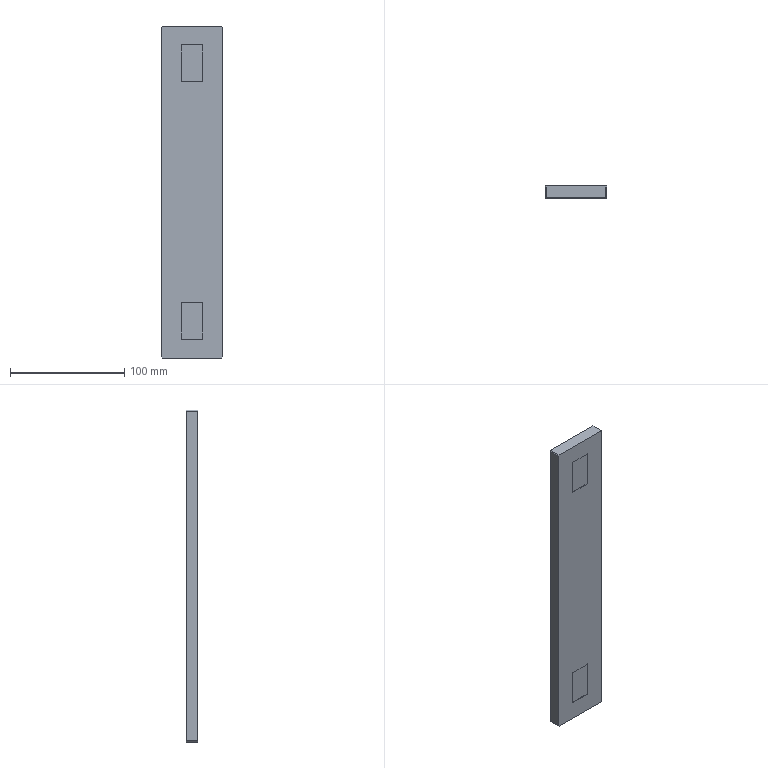Part | SolidWorks | 1 solid | 25 faces | box 54 x 10 x 290 mm | volume 145188 mm3 | plane 25
STEP:
#1=CARTESIAN_POINT('',(9.25,0.,-96.5));
#2=VERTEX_POINT('',#1);
#3=CARTESIAN_POINT('',(9.25,0.5,-96.5));
#4=VERTEX_POINT('',#3);
#5=CARTESIAN_POINT('',(9.25,-193.885,-96.5));
#6=DIRECTION('',(0.,1.,0.));
#7=VECTOR('',#6,1000.);
#8=LINE('',#5,#7);
#9=EDGE_CURVE('',#2,#4,#8,.T.);
#10=ORIENTED_EDGE('',*,*,#9,.T.);
#11=CARTESIAN_POINT('',(9.25,0.5,-128.5));
#12=VERTEX_POINT('',#11);
#13=CARTESIAN_POINT('',(9.25,0.5,128.5));
#14=DIRECTION('',(0.,0.,1.));
#15=VECTOR('',#14,1000.);
#16=LINE('',#13,#15);
#17=EDGE_CURVE('',#12,#4,#16,.T.);
#18=ORIENTED_EDGE('',*,*,#17,.F.);
#19=CARTESIAN_POINT('',(9.25,0.,-128.5));
#20=VERTEX_POINT('',#19);
#21=CARTESIAN_POINT('',(9.25,0.5,-128.5));
#22=DIRECTION('',(0.,-1.,0.));
#23=VECTOR('',#22,1000.);
#24=LINE('',#21,#23);
#25=EDGE_CURVE('',#12,#20,#24,.T.);
#26=ORIENTED_EDGE('',*,*,#25,.T.);
#27=CARTESIAN_POINT('',(9.25,0.,128.5));
#28=DIRECTION('',(0.,0.,1.));
#29=VECTOR('',#28,1000.);
#30=LINE('',#27,#29);
#31=EDGE_CURVE('',#20,#2,#30,.T.);
#32=ORIENTED_EDGE('',*,*,#31,.T.);
#33=EDGE_LOOP('',(#10,#18,#26,#32));
#34=FACE_OUTER_BOUND('',#33,.T.);
#35=CARTESIAN_POINT('',(9.25,0.5,128.5));
#36=DIRECTION('',(1.,0.,0.));
#37=DIRECTION('',(0.,0.,-1.));
#38=AXIS2_PLACEMENT_3D('',#35,#36,#37);
#39=PLANE('',#38);
#40=ADVANCED_FACE('',(#34),#39,.F.);
#41=CARTESIAN_POINT('',(9.25,0.,96.5));
#42=VERTEX_POINT('',#41);
#43=CARTESIAN_POINT('',(9.25,0.5,96.5));
#44=VERTEX_POINT('',#43);
#45=CARTESIAN_POINT('',(9.25,-193.885,96.5));
#46=DIRECTION('',(0.,1.,0.));
#47=VECTOR('',#46,1000.);
#48=LINE('',#45,#47);
#49=EDGE_CURVE('',#42,#44,#48,.T.);
#50=ORIENTED_EDGE('',*,*,#49,.F.);
#51=CARTESIAN_POINT('',(9.25,0.,128.5));
#52=VERTEX_POINT('',#51);
#53=CARTESIAN_POINT('',(9.25,0.,128.5));
#54=DIRECTION('',(0.,0.,1.));
#55=VECTOR('',#54,1000.);
#56=LINE('',#53,#55);
#57=EDGE_CURVE('',#42,#52,#56,.T.);
#58=ORIENTED_EDGE('',*,*,#57,.T.);
#59=CARTESIAN_POINT('',(9.25,0.5,128.5));
#60=VERTEX_POINT('',#59);
#61=CARTESIAN_POINT('',(9.25,0.5,128.5));
#62=DIRECTION('',(0.,-1.,0.));
#63=VECTOR('',#62,1000.);
#64=LINE('',#61,#63);
#65=EDGE_CURVE('',#60,#52,#64,.T.);
#66=ORIENTED_EDGE('',*,*,#65,.F.);
#67=CARTESIAN_POINT('',(9.25,0.5,128.5));
#68=DIRECTION('',(0.,0.,1.));
#69=VECTOR('',#68,1000.);
#70=LINE('',#67,#69);
#71=EDGE_CURVE('',#44,#60,#70,.T.);
#72=ORIENTED_EDGE('',*,*,#71,.F.);
#73=EDGE_LOOP('',(#50,#58,#66,#72));
#74=FACE_OUTER_BOUND('',#73,.T.);
#75=CARTESIAN_POINT('',(9.25,0.5,128.5));
#76=DIRECTION('',(1.,0.,0.));
#77=DIRECTION('',(0.,0.,-1.));
#78=AXIS2_PLACEMENT_3D('',#75,#76,#77);
#79=PLANE('',#78);
#80=ADVANCED_FACE('',(#74),#79,.F.);
#81=CARTESIAN_POINT('',(-9.25,0.,-96.5));
#82=VERTEX_POINT('',#81);
#83=CARTESIAN_POINT('',(-9.25,0.5,-96.5));
#84=VERTEX_POINT('',#83);
#85=CARTESIAN_POINT('',(-9.25,-193.885,-96.5));
#86=DIRECTION('',(0.,1.,0.));
#87=VECTOR('',#86,1000.);
#88=LINE('',#85,#87);
#89=EDGE_CURVE('',#82,#84,#88,.T.);
#90=ORIENTED_EDGE('',*,*,#89,.F.);
#91=CARTESIAN_POINT('',(-9.25,0.,-128.5));
#92=VERTEX_POINT('',#91);
#93=CARTESIAN_POINT('',(-9.25,0.,128.5));
#94=DIRECTION('',(0.,0.,-1.));
#95=VECTOR('',#94,1000.);
#96=LINE('',#93,#95);
#97=EDGE_CURVE('',#82,#92,#96,.T.);
#98=ORIENTED_EDGE('',*,*,#97,.T.);
#99=CARTESIAN_POINT('',(-9.25,0.5,-128.5));
#100=VERTEX_POINT('',#99);
#101=CARTESIAN_POINT('',(-9.25,0.5,-128.5));
#102=DIRECTION('',(0.,-1.,0.));
#103=VECTOR('',#102,1000.);
#104=LINE('',#101,#103);
#105=EDGE_CURVE('',#100,#92,#104,.T.);
#106=ORIENTED_EDGE('',*,*,#105,.F.);
#107=CARTESIAN_POINT('',(-9.25,0.5,128.5));
#108=DIRECTION('',(0.,0.,-1.));
#109=VECTOR('',#108,1000.);
#110=LINE('',#107,#109);
#111=EDGE_CURVE('',#84,#100,#110,.T.);
#112=ORIENTED_EDGE('',*,*,#111,.F.);
#113=EDGE_LOOP('',(#90,#98,#106,#112));
#114=FACE_OUTER_BOUND('',#113,.T.);
#115=CARTESIAN_POINT('',(-9.25,0.5,128.5));
#116=DIRECTION('',(-1.,0.,0.));
#117=DIRECTION('',(0.,0.,1.));
#118=AXIS2_PLACEMENT_3D('',#115,#116,#117);
#119=PLANE('',#118);
#120=ADVANCED_FACE('',(#114),#119,.F.);
#121=CARTESIAN_POINT('',(-9.25,0.,96.5));
#122=VERTEX_POINT('',#121);
#123=CARTESIAN_POINT('',(-9.25,0.5,96.5));
#124=VERTEX_POINT('',#123);
#125=CARTESIAN_POINT('',(-9.25,-193.885,96.5));
#126=DIRECTION('',(0.,1.,0.));
#127=VECTOR('',#126,1000.);
#128=LINE('',#125,#127);
#129=EDGE_CURVE('',#122,#124,#128,.T.);
#130=ORIENTED_EDGE('',*,*,#129,.T.);
#131=CARTESIAN_POINT('',(-9.25,0.5,128.5));
#132=VERTEX_POINT('',#131);
#133=CARTESIAN_POINT('',(-9.25,0.5,128.5));
#134=DIRECTION('',(0.,0.,-1.));
#135=VECTOR('',#134,1000.);
#136=LINE('',#133,#135);
#137=EDGE_CURVE('',#132,#124,#136,.T.);
#138=ORIENTED_EDGE('',*,*,#137,.F.);
#139=CARTESIAN_POINT('',(-9.25,0.,128.5));
#140=VERTEX_POINT('',#139);
#141=CARTESIAN_POINT('',(-9.25,0.5,128.5));
#142=DIRECTION('',(0.,-1.,0.));
#143=VECTOR('',#142,1000.);
#144=LINE('',#141,#143);
#145=EDGE_CURVE('',#132,#140,#144,.T.);
#146=ORIENTED_EDGE('',*,*,#145,.T.);
#147=CARTESIAN_POINT('',(-9.25,0.,128.5));
#148=DIRECTION('',(0.,0.,-1.));
#149=VECTOR('',#148,1000.);
#150=LINE('',#147,#149);
#151=EDGE_CURVE('',#140,#122,#150,.T.);
#152=ORIENTED_EDGE('',*,*,#151,.T.);
#153=EDGE_LOOP('',(#130,#138,#146,#152));
#154=FACE_OUTER_BOUND('',#153,.T.);
#155=CARTESIAN_POINT('',(-9.25,0.5,128.5));
#156=DIRECTION('',(-1.,0.,0.));
#157=DIRECTION('',(0.,0.,1.));
#158=AXIS2_PLACEMENT_3D('',#155,#156,#157);
#159=PLANE('',#158);
#160=ADVANCED_FACE('',(#154),#159,.F.);
#161=ORIENTED_EDGE('',*,*,#17,.T.);
#162=CARTESIAN_POINT('',(-9.25,0.5,-96.5));
#163=DIRECTION('',(1.,0.,0.));
#164=VECTOR('',#163,1000.);
#165=LINE('',#162,#164);
#166=EDGE_CURVE('',#84,#4,#165,.T.);
#167=ORIENTED_EDGE('',*,*,#166,.F.);
#168=ORIENTED_EDGE('',*,*,#111,.T.);
#169=CARTESIAN_POINT('',(-9.25,0.5,-128.5));
#170=DIRECTION('',(1.,0.,0.));
#171=VECTOR('',#170,1000.);
#172=LINE('',#169,#171);
#173=EDGE_CURVE('',#100,#12,#172,.T.);
#174=ORIENTED_EDGE('',*,*,#173,.T.);
#175=EDGE_LOOP('',(#161,#167,#168,#174));
#176=FACE_OUTER_BOUND('',#175,.T.);
#177=CARTESIAN_POINT('',(0.,0.5,0.));
#178=DIRECTION('',(0.,-1.,0.));
#179=DIRECTION('',(0.,0.,-1.));
#180=AXIS2_PLACEMENT_3D('',#177,#178,#179);
#181=PLANE('',#180);
#182=ADVANCED_FACE('',(#176),#181,.T.);
#183=ORIENTED_EDGE('',*,*,#137,.T.);
#184=CARTESIAN_POINT('',(-9.25,0.5,96.5));
#185=DIRECTION('',(-1.,0.,0.));
#186=VECTOR('',#185,1000.);
#187=LINE('',#184,#186);
#188=EDGE_CURVE('',#44,#124,#187,.T.);
#189=ORIENTED_EDGE('',*,*,#188,.F.);
#190=ORIENTED_EDGE('',*,*,#71,.T.);
#191=CARTESIAN_POINT('',(-9.25,0.5,128.5));
#192=DIRECTION('',(-1.,0.,0.));
#193=VECTOR('',#192,1000.);
#194=LINE('',#191,#193);
#195=EDGE_CURVE('',#60,#132,#194,.T.);
#196=ORIENTED_EDGE('',*,*,#195,.T.);
#197=EDGE_LOOP('',(#183,#189,#190,#196));
#198=FACE_OUTER_BOUND('',#197,.T.);
#199=CARTESIAN_POINT('',(0.,0.5,0.));
#200=DIRECTION('',(0.,-1.,0.));
#201=DIRECTION('',(0.,0.,-1.));
#202=AXIS2_PLACEMENT_3D('',#199,#200,#201);
#203=PLANE('',#202);
#204=ADVANCED_FACE('',(#198),#203,.T.);
#205=CARTESIAN_POINT('',(27.,0.,144.));
#206=VERTEX_POINT('',#205);
#207=CARTESIAN_POINT('',(27.,0.,-144.));
#208=VERTEX_POINT('',#207);
#209=CARTESIAN_POINT('',(27.,0.,-145.));
#210=DIRECTION('',(0.,0.,-1.));
#211=VECTOR('',#210,1000.);
#212=LINE('',#209,#211);
#213=EDGE_CURVE('',#206,#208,#212,.T.);
#214=ORIENTED_EDGE('',*,*,#213,.T.);
#215=CARTESIAN_POINT('',(27.,10.,-144.));
#216=VERTEX_POINT('',#215);
#217=CARTESIAN_POINT('',(27.,10.,-144.));
#218=DIRECTION('',(0.,1.,0.));
#219=VECTOR('',#218,1000.);
#220=LINE('',#217,#219);
#221=EDGE_CURVE('',#208,#216,#220,.T.);
#222=ORIENTED_EDGE('',*,*,#221,.T.);
#223=CARTESIAN_POINT('',(27.,10.,144.));
#224=VERTEX_POINT('',#223);
#225=CARTESIAN_POINT('',(27.,10.,-145.));
#226=DIRECTION('',(0.,0.,-1.));
#227=VECTOR('',#226,1000.);
#228=LINE('',#225,#227);
#229=EDGE_CURVE('',#224,#216,#228,.T.);
#230=ORIENTED_EDGE('',*,*,#229,.F.);
#231=CARTESIAN_POINT('',(27.,10.,144.));
#232=DIRECTION('',(0.,-1.,0.));
#233=VECTOR('',#232,1000.);
#234=LINE('',#231,#233);
#235=EDGE_CURVE('',#224,#206,#234,.T.);
#236=ORIENTED_EDGE('',*,*,#235,.T.);
#237=EDGE_LOOP('',(#214,#222,#230,#236));
#238=FACE_OUTER_BOUND('',#237,.T.);
#239=CARTESIAN_POINT('',(27.,10.,-145.));
#240=DIRECTION('',(-1.,0.,0.));
#241=DIRECTION('',(0.,0.,1.));
#242=AXIS2_PLACEMENT_3D('',#239,#240,#241);
#243=PLANE('',#242);
#244=ADVANCED_FACE('',(#238),#243,.F.);
#245=CARTESIAN_POINT('',(26.,10.,-145.));
#246=VERTEX_POINT('',#245);
#247=CARTESIAN_POINT('',(-26.,10.,-145.));
#248=VERTEX_POINT('',#247);
#249=CARTESIAN_POINT('',(-27.,10.,-145.));
#250=DIRECTION('',(-1.,0.,0.));
#251=VECTOR('',#250,1000.);
#252=LINE('',#249,#251);
#253=EDGE_CURVE('',#246,#248,#252,.T.);
#254=ORIENTED_EDGE('',*,*,#253,.F.);
#255=CARTESIAN_POINT('',(26.,0.,-145.));
#256=VERTEX_POINT('',#255);
#257=CARTESIAN_POINT('',(26.,10.,-145.));
#258=DIRECTION('',(0.,-1.,0.));
#259=VECTOR('',#258,1000.);
#260=LINE('',#257,#259);
#261=EDGE_CURVE('',#246,#256,#260,.T.);
#262=ORIENTED_EDGE('',*,*,#261,.T.);
#263=CARTESIAN_POINT('',(-26.,0.,-145.));
#264=VERTEX_POINT('',#263);
#265=CARTESIAN_POINT('',(-27.,0.,-145.));
#266=DIRECTION('',(-1.,0.,0.));
#267=VECTOR('',#266,1000.);
#268=LINE('',#265,#267);
#269=EDGE_CURVE('',#256,#264,#268,.T.);
#270=ORIENTED_EDGE('',*,*,#269,.T.);
#271=CARTESIAN_POINT('',(-26.,10.,-145.));
#272=DIRECTION('',(0.,1.,0.));
#273=VECTOR('',#272,1000.);
#274=LINE('',#271,#273);
#275=EDGE_CURVE('',#264,#248,#274,.T.);
#276=ORIENTED_EDGE('',*,*,#275,.T.);
#277=EDGE_LOOP('',(#254,#262,#270,#276));
#278=FACE_OUTER_BOUND('',#277,.T.);
#279=CARTESIAN_POINT('',(-27.,10.,-145.));
#280=DIRECTION('',(0.,0.,1.));
#281=DIRECTION('',(1.,0.,0.));
#282=AXIS2_PLACEMENT_3D('',#279,#280,#281);
#283=PLANE('',#282);
#284=ADVANCED_FACE('',(#278),#283,.F.);
#285=CARTESIAN_POINT('',(-27.,10.,-144.));
#286=VERTEX_POINT('',#285);
#287=CARTESIAN_POINT('',(-27.,10.,144.));
#288=VERTEX_POINT('',#287);
#289=CARTESIAN_POINT('',(-27.,10.,-145.));
#290=DIRECTION('',(0.,0.,1.));
#291=VECTOR('',#290,1000.);
#292=LINE('',#289,#291);
#293=EDGE_CURVE('',#286,#288,#292,.T.);
#294=ORIENTED_EDGE('',*,*,#293,.F.);
#295=CARTESIAN_POINT('',(-27.,0.,-144.));
#296=VERTEX_POINT('',#295);
#297=CARTESIAN_POINT('',(-27.,10.,-144.));
#298=DIRECTION('',(0.,-1.,0.));
#299=VECTOR('',#298,1000.);
#300=LINE('',#297,#299);
#301=EDGE_CURVE('',#286,#296,#300,.T.);
#302=ORIENTED_EDGE('',*,*,#301,.T.);
#303=CARTESIAN_POINT('',(-27.,0.,144.));
#304=VERTEX_POINT('',#303);
#305=CARTESIAN_POINT('',(-27.,0.,-145.));
#306=DIRECTION('',(0.,0.,1.));
#307=VECTOR('',#306,1000.);
#308=LINE('',#305,#307);
#309=EDGE_CURVE('',#296,#304,#308,.T.);
#310=ORIENTED_EDGE('',*,*,#309,.T.);
#311=CARTESIAN_POINT('',(-27.,10.,144.));
#312=DIRECTION('',(0.,1.,0.));
#313=VECTOR('',#312,1000.);
#314=LINE('',#311,#313);
#315=EDGE_CURVE('',#304,#288,#314,.T.);
#316=ORIENTED_EDGE('',*,*,#315,.T.);
#317=EDGE_LOOP('',(#294,#302,#310,#316));
#318=FACE_OUTER_BOUND('',#317,.T.);
#319=CARTESIAN_POINT('',(-27.,10.,-145.));
#320=DIRECTION('',(1.,0.,0.));
#321=DIRECTION('',(0.,0.,-1.));
#322=AXIS2_PLACEMENT_3D('',#319,#320,#321);
#323=PLANE('',#322);
#324=ADVANCED_FACE('',(#318),#323,.F.);
#325=CARTESIAN_POINT('',(-26.,0.,145.));
#326=VERTEX_POINT('',#325);
#327=CARTESIAN_POINT('',(26.,0.,145.));
#328=VERTEX_POINT('',#327);
#329=CARTESIAN_POINT('',(-27.,0.,145.));
#330=DIRECTION('',(1.,0.,0.));
#331=VECTOR('',#330,1000.);
#332=LINE('',#329,#331);
#333=EDGE_CURVE('',#326,#328,#332,.T.);
#334=ORIENTED_EDGE('',*,*,#333,.T.);
#335=CARTESIAN_POINT('',(26.,10.,145.));
#336=VERTEX_POINT('',#335);
#337=CARTESIAN_POINT('',(26.,10.,145.));
#338=DIRECTION('',(0.,1.,0.));
#339=VECTOR('',#338,1000.);
#340=LINE('',#337,#339);
#341=EDGE_CURVE('',#328,#336,#340,.T.);
#342=ORIENTED_EDGE('',*,*,#341,.T.);
#343=CARTESIAN_POINT('',(-26.,10.,145.));
#344=VERTEX_POINT('',#343);
#345=CARTESIAN_POINT('',(-27.,10.,145.));
#346=DIRECTION('',(1.,0.,0.));
#347=VECTOR('',#346,1000.);
#348=LINE('',#345,#347);
#349=EDGE_CURVE('',#344,#336,#348,.T.);
#350=ORIENTED_EDGE('',*,*,#349,.F.);
#351=CARTESIAN_POINT('',(-26.,10.,145.));
#352=DIRECTION('',(0.,-1.,0.));
#353=VECTOR('',#352,1000.);
#354=LINE('',#351,#353);
#355=EDGE_CURVE('',#344,#326,#354,.T.);
#356=ORIENTED_EDGE('',*,*,#355,.T.);
#357=EDGE_LOOP('',(#334,#342,#350,#356));
#358=FACE_OUTER_BOUND('',#357,.T.);
#359=CARTESIAN_POINT('',(-27.,10.,145.));
#360=DIRECTION('',(0.,0.,-1.));
#361=DIRECTION('',(-1.,0.,0.));
#362=AXIS2_PLACEMENT_3D('',#359,#360,#361);
#363=PLANE('',#362);
#364=ADVANCED_FACE('',(#358),#363,.F.);
#365=CARTESIAN_POINT('',(-7.5,10.,120.));
#366=VERTEX_POINT('',#365);
#367=CARTESIAN_POINT('',(-7.5,10.,-120.));
#368=VERTEX_POINT('',#367);
#369=CARTESIAN_POINT('',(-7.5,10.,-120.));
#370=DIRECTION('',(0.,0.,-1.));
#371=VECTOR('',#370,1000.);
#372=LINE('',#369,#371);
#373=EDGE_CURVE('',#366,#368,#372,.T.);
#374=ORIENTED_EDGE('',*,*,#373,.F.);
#375=CARTESIAN_POINT('',(-22.5,10.,120.));
#376=VERTEX_POINT('',#375);
#377=CARTESIAN_POINT('',(-22.5,10.,120.));
#378=DIRECTION('',(1.,0.,0.));
#379=VECTOR('',#378,1000.);
#380=LINE('',#377,#379);
#381=EDGE_CURVE('',#376,#366,#380,.T.);
#382=ORIENTED_EDGE('',*,*,#381,.F.);
#383=CARTESIAN_POINT('',(-22.5,10.,-120.));
#384=VERTEX_POINT('',#383);
#385=CARTESIAN_POINT('',(-22.5,10.,-120.));
#386=DIRECTION('',(0.,0.,1.));
#387=VECTOR('',#386,1000.);
#388=LINE('',#385,#387);
#389=EDGE_CURVE('',#384,#376,#388,.T.);
#390=ORIENTED_EDGE('',*,*,#389,.F.);
#391=CARTESIAN_POINT('',(-22.5,10.,-120.));
#392=DIRECTION('',(-1.,0.,0.));
#393=VECTOR('',#392,1000.);
#394=LINE('',#391,#393);
#395=EDGE_CURVE('',#368,#384,#394,.T.);
#396=ORIENTED_EDGE('',*,*,#395,.F.);
#397=EDGE_LOOP('',(#374,#382,#390,#396));
#398=FACE_BOUND('',#397,.T.);
#399=ORIENTED_EDGE('',*,*,#229,.T.);
#400=CARTESIAN_POINT('',(85.5,10.,-85.5));
#401=DIRECTION('',(-0.7071,0.,-0.7071));
#402=VECTOR('',#401,1000.);
#403=LINE('',#400,#402);
#404=EDGE_CURVE('',#216,#246,#403,.T.);
#405=ORIENTED_EDGE('',*,*,#404,.T.);
#406=ORIENTED_EDGE('',*,*,#253,.T.);
#407=CARTESIAN_POINT('',(-85.5,10.,-85.5));
#408=DIRECTION('',(-0.7071,0.,0.7071));
#409=VECTOR('',#408,1000.);
#410=LINE('',#407,#409);
#411=EDGE_CURVE('',#248,#286,#410,.T.);
#412=ORIENTED_EDGE('',*,*,#411,.T.);
#413=ORIENTED_EDGE('',*,*,#293,.T.);
#414=CARTESIAN_POINT('',(-85.5,10.,85.5));
#415=DIRECTION('',(0.7071,0.,0.7071));
#416=VECTOR('',#415,1000.);
#417=LINE('',#414,#416);
#418=EDGE_CURVE('',#288,#344,#417,.T.);
#419=ORIENTED_EDGE('',*,*,#418,.T.);
#420=ORIENTED_EDGE('',*,*,#349,.T.);
#421=CARTESIAN_POINT('',(85.5,10.,85.5));
#422=DIRECTION('',(0.7071,0.,-0.7071));
#423=VECTOR('',#422,1000.);
#424=LINE('',#421,#423);
#425=EDGE_CURVE('',#336,#224,#424,.T.);
#426=ORIENTED_EDGE('',*,*,#425,.T.);
#427=EDGE_LOOP('',(#399,#405,#406,#412,#413,#419,#420,#426));
#428=FACE_OUTER_BOUND('',#427,.T.);
#429=CARTESIAN_POINT('',(0.,10.,0.));
#430=DIRECTION('',(0.,1.,0.));
#431=DIRECTION('',(0.,0.,1.));
#432=AXIS2_PLACEMENT_3D('',#429,#430,#431);
#433=PLANE('',#432);
#434=ADVANCED_FACE('',(#398,#428),#433,.T.);
#435=CARTESIAN_POINT('',(-9.25,0.,-96.5));
#436=DIRECTION('',(-1.,0.,0.));
#437=VECTOR('',#436,1000.);
#438=LINE('',#435,#437);
#439=EDGE_CURVE('',#2,#82,#438,.T.);
#440=ORIENTED_EDGE('',*,*,#439,.F.);
#441=ORIENTED_EDGE('',*,*,#31,.F.);
#442=CARTESIAN_POINT('',(-9.25,0.,-128.5));
#443=DIRECTION('',(1.,0.,0.));
#444=VECTOR('',#443,1000.);
#445=LINE('',#442,#444);
#446=EDGE_CURVE('',#92,#20,#445,.T.);
#447=ORIENTED_EDGE('',*,*,#446,.F.);
#448=ORIENTED_EDGE('',*,*,#97,.F.);
#449=EDGE_LOOP('',(#440,#441,#447,#448));
#450=FACE_BOUND('',#449,.T.);
#451=CARTESIAN_POINT('',(-9.25,0.,128.5));
#452=DIRECTION('',(-1.,0.,0.));
#453=VECTOR('',#452,1000.);
#454=LINE('',#451,#453);
#455=EDGE_CURVE('',#52,#140,#454,.T.);
#456=ORIENTED_EDGE('',*,*,#455,.F.);
#457=ORIENTED_EDGE('',*,*,#57,.F.);
#458=CARTESIAN_POINT('',(-9.25,0.,96.5));
#459=DIRECTION('',(1.,0.,0.));
#460=VECTOR('',#459,1000.);
#461=LINE('',#458,#460);
#462=EDGE_CURVE('',#122,#42,#461,.T.);
#463=ORIENTED_EDGE('',*,*,#462,.F.);
#464=ORIENTED_EDGE('',*,*,#151,.F.);
#465=EDGE_LOOP('',(#456,#457,#463,#464));
#466=FACE_BOUND('',#465,.T.);
#467=ORIENTED_EDGE('',*,*,#269,.F.);
#468=CARTESIAN_POINT('',(26.,0.,-145.));
#469=DIRECTION('',(0.7071,0.,0.7071));
#470=VECTOR('',#469,1000.);
#471=LINE('',#468,#470);
#472=EDGE_CURVE('',#256,#208,#471,.T.);
#473=ORIENTED_EDGE('',*,*,#472,.T.);
#474=ORIENTED_EDGE('',*,*,#213,.F.);
#475=CARTESIAN_POINT('',(27.,0.,144.));
#476=DIRECTION('',(-0.7071,0.,0.7071));
#477=VECTOR('',#476,1000.);
#478=LINE('',#475,#477);
#479=EDGE_CURVE('',#206,#328,#478,.T.);
#480=ORIENTED_EDGE('',*,*,#479,.T.);
#481=ORIENTED_EDGE('',*,*,#333,.F.);
#482=CARTESIAN_POINT('',(-26.,0.,145.));
#483=DIRECTION('',(-0.7071,0.,-0.7071));
#484=VECTOR('',#483,1000.);
#485=LINE('',#482,#484);
#486=EDGE_CURVE('',#326,#304,#485,.T.);
#487=ORIENTED_EDGE('',*,*,#486,.T.);
#488=ORIENTED_EDGE('',*,*,#309,.F.);
#489=CARTESIAN_POINT('',(-27.,0.,-144.));
#490=DIRECTION('',(0.7071,0.,-0.7071));
#491=VECTOR('',#490,1000.);
#492=LINE('',#489,#491);
#493=EDGE_CURVE('',#296,#264,#492,.T.);
#494=ORIENTED_EDGE('',*,*,#493,.T.);
#495=EDGE_LOOP('',(#467,#473,#474,#480,#481,#487,#488,#494));
#496=FACE_OUTER_BOUND('',#495,.T.);
#497=CARTESIAN_POINT('',(0.,0.,0.));
#498=DIRECTION('',(0.,1.,0.));
#499=DIRECTION('',(0.,0.,1.));
#500=AXIS2_PLACEMENT_3D('',#497,#498,#499);
#501=PLANE('',#500);
#502=ADVANCED_FACE('',(#450,#466,#496),#501,.F.);
#503=ORIENTED_EDGE('',*,*,#446,.T.);
#504=ORIENTED_EDGE('',*,*,#25,.F.);
#505=ORIENTED_EDGE('',*,*,#173,.F.);
#506=ORIENTED_EDGE('',*,*,#105,.T.);
#507=EDGE_LOOP('',(#503,#504,#505,#506));
#508=FACE_OUTER_BOUND('',#507,.T.);
#509=CARTESIAN_POINT('',(-9.25,0.5,-128.5));
#510=DIRECTION('',(0.,0.,-1.));
#511=DIRECTION('',(-1.,0.,0.));
#512=AXIS2_PLACEMENT_3D('',#509,#510,#511);
#513=PLANE('',#512);
#514=ADVANCED_FACE('',(#508),#513,.F.);
#515=ORIENTED_EDGE('',*,*,#455,.T.);
#516=ORIENTED_EDGE('',*,*,#145,.F.);
#517=ORIENTED_EDGE('',*,*,#195,.F.);
#518=ORIENTED_EDGE('',*,*,#65,.T.);
#519=EDGE_LOOP('',(#515,#516,#517,#518));
#520=FACE_OUTER_BOUND('',#519,.T.);
#521=CARTESIAN_POINT('',(-9.25,0.5,128.5));
#522=DIRECTION('',(0.,0.,1.));
#523=DIRECTION('',(1.,0.,0.));
#524=AXIS2_PLACEMENT_3D('',#521,#522,#523);
#525=PLANE('',#524);
#526=ADVANCED_FACE('',(#520),#525,.F.);
#527=ORIENTED_EDGE('',*,*,#9,.F.);
#528=ORIENTED_EDGE('',*,*,#439,.T.);
#529=ORIENTED_EDGE('',*,*,#89,.T.);
#530=ORIENTED_EDGE('',*,*,#166,.T.);
#531=EDGE_LOOP('',(#527,#528,#529,#530));
#532=FACE_OUTER_BOUND('',#531,.T.);
#533=CARTESIAN_POINT('',(-9.25,-193.885,-96.5));
#534=DIRECTION('',(0.,0.,1.));
#535=DIRECTION('',(1.,0.,0.));
#536=AXIS2_PLACEMENT_3D('',#533,#534,#535);
#537=PLANE('',#536);
#538=ADVANCED_FACE('',(#532),#537,.F.);
#539=ORIENTED_EDGE('',*,*,#129,.F.);
#540=ORIENTED_EDGE('',*,*,#462,.T.);
#541=ORIENTED_EDGE('',*,*,#49,.T.);
#542=ORIENTED_EDGE('',*,*,#188,.T.);
#543=EDGE_LOOP('',(#539,#540,#541,#542));
#544=FACE_OUTER_BOUND('',#543,.T.);
#545=CARTESIAN_POINT('',(-9.25,-193.885,96.5));
#546=DIRECTION('',(0.,0.,-1.));
#547=DIRECTION('',(-1.,0.,0.));
#548=AXIS2_PLACEMENT_3D('',#545,#546,#547);
#549=PLANE('',#548);
#550=ADVANCED_FACE('',(#544),#549,.F.);
#551=ORIENTED_EDGE('',*,*,#404,.F.);
#552=ORIENTED_EDGE('',*,*,#221,.F.);
#553=ORIENTED_EDGE('',*,*,#472,.F.);
#554=ORIENTED_EDGE('',*,*,#261,.F.);
#555=EDGE_LOOP('',(#551,#552,#553,#554));
#556=FACE_OUTER_BOUND('',#555,.T.);
#557=CARTESIAN_POINT('',(26.,10.,-145.));
#558=DIRECTION('',(-0.7071,0.,0.7071));
#559=DIRECTION('',(0.,-1.,0.));
#560=AXIS2_PLACEMENT_3D('',#557,#558,#559);
#561=PLANE('',#560);
#562=ADVANCED_FACE('',(#556),#561,.F.);
#563=ORIENTED_EDGE('',*,*,#411,.F.);
#564=ORIENTED_EDGE('',*,*,#275,.F.);
#565=ORIENTED_EDGE('',*,*,#493,.F.);
#566=ORIENTED_EDGE('',*,*,#301,.F.);
#567=EDGE_LOOP('',(#563,#564,#565,#566));
#568=FACE_OUTER_BOUND('',#567,.T.);
#569=CARTESIAN_POINT('',(-27.,10.,-144.));
#570=DIRECTION('',(0.7071,0.,0.7071));
#571=DIRECTION('',(0.,-1.,0.));
#572=AXIS2_PLACEMENT_3D('',#569,#570,#571);
#573=PLANE('',#572);
#574=ADVANCED_FACE('',(#568),#573,.F.);
#575=ORIENTED_EDGE('',*,*,#425,.F.);
#576=ORIENTED_EDGE('',*,*,#341,.F.);
#577=ORIENTED_EDGE('',*,*,#479,.F.);
#578=ORIENTED_EDGE('',*,*,#235,.F.);
#579=EDGE_LOOP('',(#575,#576,#577,#578));
#580=FACE_OUTER_BOUND('',#579,.T.);
#581=CARTESIAN_POINT('',(27.,10.,144.));
#582=DIRECTION('',(-0.7071,0.,-0.7071));
#583=DIRECTION('',(0.,-1.,0.));
#584=AXIS2_PLACEMENT_3D('',#581,#582,#583);
#585=PLANE('',#584);
#586=ADVANCED_FACE('',(#580),#585,.F.);
#587=ORIENTED_EDGE('',*,*,#418,.F.);
#588=ORIENTED_EDGE('',*,*,#315,.F.);
#589=ORIENTED_EDGE('',*,*,#486,.F.);
#590=ORIENTED_EDGE('',*,*,#355,.F.);
#591=EDGE_LOOP('',(#587,#588,#589,#590));
#592=FACE_OUTER_BOUND('',#591,.T.);
#593=CARTESIAN_POINT('',(-26.,10.,145.));
#594=DIRECTION('',(0.7071,0.,-0.7071));
#595=DIRECTION('',(0.,-1.,0.));
#596=AXIS2_PLACEMENT_3D('',#593,#594,#595);
#597=PLANE('',#596);
#598=ADVANCED_FACE('',(#592),#597,.F.);
#599=ORIENTED_EDGE('',*,*,#373,.T.);
#600=CARTESIAN_POINT('',(-7.5,7.,-120.));
#601=VERTEX_POINT('',#600);
#602=CARTESIAN_POINT('',(-7.5,7.,-120.));
#603=DIRECTION('',(0.,1.,0.));
#604=VECTOR('',#603,1000.);
#605=LINE('',#602,#604);
#606=EDGE_CURVE('',#601,#368,#605,.T.);
#607=ORIENTED_EDGE('',*,*,#606,.F.);
#608=CARTESIAN_POINT('',(-7.5,7.,120.));
#609=VERTEX_POINT('',#608);
#610=CARTESIAN_POINT('',(-7.5,7.,-120.));
#611=DIRECTION('',(0.,0.,-1.));
#612=VECTOR('',#611,1000.);
#613=LINE('',#610,#612);
#614=EDGE_CURVE('',#609,#601,#613,.T.);
#615=ORIENTED_EDGE('',*,*,#614,.F.);
#616=CARTESIAN_POINT('',(-7.5,7.,120.));
#617=DIRECTION('',(0.,1.,0.));
#618=VECTOR('',#617,1000.);
#619=LINE('',#616,#618);
#620=EDGE_CURVE('',#609,#366,#619,.T.);
#621=ORIENTED_EDGE('',*,*,#620,.T.);
#622=EDGE_LOOP('',(#599,#607,#615,#621));
#623=FACE_OUTER_BOUND('',#622,.T.);
#624=CARTESIAN_POINT('',(-7.5,7.,-120.));
#625=DIRECTION('',(1.,0.,0.));
#626=DIRECTION('',(0.,0.,-1.));
#627=AXIS2_PLACEMENT_3D('',#624,#625,#626);
#628=PLANE('',#627);
#629=ADVANCED_FACE('',(#623),#628,.F.);
#630=ORIENTED_EDGE('',*,*,#381,.T.);
#631=ORIENTED_EDGE('',*,*,#620,.F.);
#632=CARTESIAN_POINT('',(-22.5,7.,120.));
#633=VERTEX_POINT('',#632);
#634=CARTESIAN_POINT('',(-22.5,7.,120.));
#635=DIRECTION('',(1.,0.,0.));
#636=VECTOR('',#635,1000.);
#637=LINE('',#634,#636);
#638=EDGE_CURVE('',#633,#609,#637,.T.);
#639=ORIENTED_EDGE('',*,*,#638,.F.);
#640=CARTESIAN_POINT('',(-22.5,7.,120.));
#641=DIRECTION('',(0.,1.,0.));
#642=VECTOR('',#641,1000.);
#643=LINE('',#640,#642);
#644=EDGE_CURVE('',#633,#376,#643,.T.);
#645=ORIENTED_EDGE('',*,*,#644,.T.);
#646=EDGE_LOOP('',(#630,#631,#639,#645));
#647=FACE_OUTER_BOUND('',#646,.T.);
#648=CARTESIAN_POINT('',(-22.5,7.,120.));
#649=DIRECTION('',(0.,0.,1.));
#650=DIRECTION('',(1.,0.,0.));
#651=AXIS2_PLACEMENT_3D('',#648,#649,#650);
#652=PLANE('',#651);
#653=ADVANCED_FACE('',(#647),#652,.F.);
#654=ORIENTED_EDGE('',*,*,#389,.T.);
#655=ORIENTED_EDGE('',*,*,#644,.F.);
#656=CARTESIAN_POINT('',(-22.5,7.,-120.));
#657=VERTEX_POINT('',#656);
#658=CARTESIAN_POINT('',(-22.5,7.,-120.));
#659=DIRECTION('',(0.,0.,1.));
#660=VECTOR('',#659,1000.);
#661=LINE('',#658,#660);
#662=EDGE_CURVE('',#657,#633,#661,.T.);
#663=ORIENTED_EDGE('',*,*,#662,.F.);
#664=CARTESIAN_POINT('',(-22.5,7.,-120.));
#665=DIRECTION('',(0.,1.,0.));
#666=VECTOR('',#665,1000.);
#667=LINE('',#664,#666);
#668=EDGE_CURVE('',#657,#384,#667,.T.);
#669=ORIENTED_EDGE('',*,*,#668,.T.);
#670=EDGE_LOOP('',(#654,#655,#663,#669));
#671=FACE_OUTER_BOUND('',#670,.T.);
#672=CARTESIAN_POINT('',(-22.5,7.,-120.));
#673=DIRECTION('',(-1.,0.,0.));
#674=DIRECTION('',(0.,0.,1.));
#675=AXIS2_PLACEMENT_3D('',#672,#673,#674);
#676=PLANE('',#675);
#677=ADVANCED_FACE('',(#671),#676,.F.);
#678=ORIENTED_EDGE('',*,*,#395,.T.);
#679=ORIENTED_EDGE('',*,*,#668,.F.);
#680=CARTESIAN_POINT('',(-22.5,7.,-120.));
#681=DIRECTION('',(-1.,0.,0.));
#682=VECTOR('',#681,1000.);
#683=LINE('',#680,#682);
#684=EDGE_CURVE('',#601,#657,#683,.T.);
#685=ORIENTED_EDGE('',*,*,#684,.F.);
#686=ORIENTED_EDGE('',*,*,#606,.T.);
#687=EDGE_LOOP('',(#678,#679,#685,#686));
#688=FACE_OUTER_BOUND('',#687,.T.);
#689=CARTESIAN_POINT('',(-22.5,7.,-120.));
#690=DIRECTION('',(0.,0.,-1.));
#691=DIRECTION('',(-1.,0.,0.));
#692=AXIS2_PLACEMENT_3D('',#689,#690,#691);
#693=PLANE('',#692);
#694=ADVANCED_FACE('',(#688),#693,.F.);
#695=ORIENTED_EDGE('',*,*,#614,.T.);
#696=ORIENTED_EDGE('',*,*,#684,.T.);
#697=ORIENTED_EDGE('',*,*,#662,.T.);
#698=ORIENTED_EDGE('',*,*,#638,.T.);
#699=EDGE_LOOP('',(#695,#696,#697,#698));
#700=FACE_OUTER_BOUND('',#699,.T.);
#701=CARTESIAN_POINT('',(0.,7.,0.));
#702=DIRECTION('',(0.,1.,0.));
#703=DIRECTION('',(0.,0.,1.));
#704=AXIS2_PLACEMENT_3D('',#701,#702,#703);
#705=PLANE('',#704);
#706=ADVANCED_FACE('',(#700),#705,.T.);
#707=CLOSED_SHELL('',(#40,#80,#120,#160,#182,#204,#244,#284,#324,#364,#434,#502,#514,#526,#538,#550,#562,#574,#586,#598,#629,#653,#677,#694,#706));
#708=MANIFOLD_SOLID_BREP('',#707);
#709=CARTESIAN_POINT('',(0.,0.,0.));
#710=DIRECTION('',(0.,0.,1.));
#711=DIRECTION('',(1.,0.,0.));
#712=AXIS2_PLACEMENT_3D('',#709,#710,#711);
#713=(LENGTH_UNIT()NAMED_UNIT(*)SI_UNIT(.MILLI.,.METRE.));
#714=UNCERTAINTY_MEASURE_WITH_UNIT(LENGTH_MEASURE(0.00001),#713,'','');
#715=(NAMED_UNIT(*)PLANE_ANGLE_UNIT()SI_UNIT($,.RADIAN.));
#716=(NAMED_UNIT(*)SI_UNIT($,.STERADIAN.)SOLID_ANGLE_UNIT());
#717=(GEOMETRIC_REPRESENTATION_CONTEXT(3)GLOBAL_UNCERTAINTY_ASSIGNED_CONTEXT((#714))GLOBAL_UNIT_ASSIGNED_CONTEXT((#713,#715,#716))REPRESENTATION_CONTEXT('',''));
#718=ADVANCED_BREP_SHAPE_REPRESENTATION('',(#708,#712),#717);